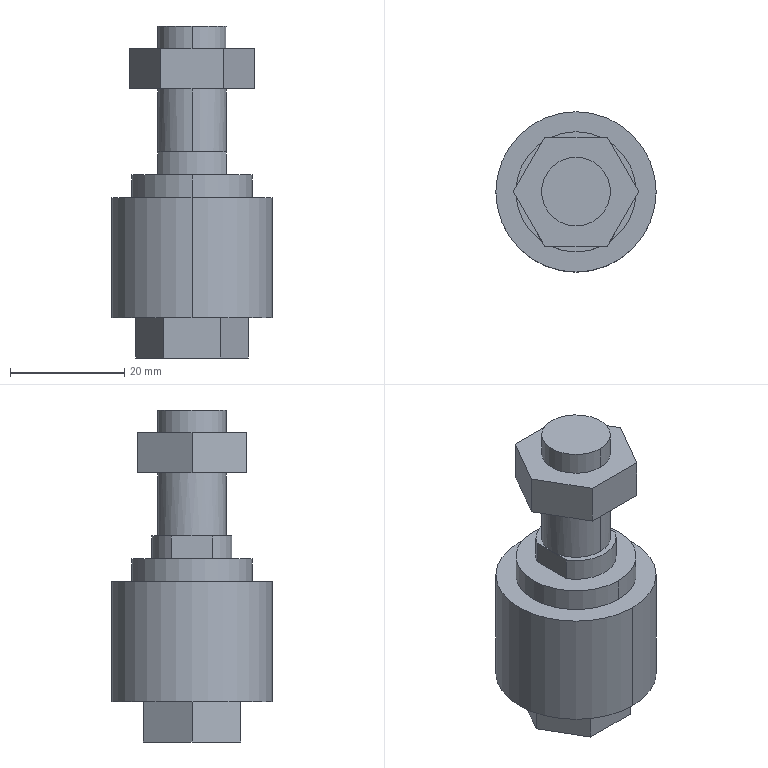Part | SolidWorks | features BaseBody 1 | 1 solid | 37 faces | box 28 x 28 x 58 mm | volume 19476 mm3 | plane 24 | cylinder 13 | commonest cylinder face diameters 12 x4 14 x3 10.8 x2 21 x2 28 x2
STEP:
#1=CARTESIAN_POINT('',(-5.4,0.,11.5));
#2=VERTEX_POINT('',#1);
#3=CARTESIAN_POINT('',(5.4,0.,11.5));
#4=VERTEX_POINT('',#3);
#5=CARTESIAN_POINT('',(0.,0.,11.5));
#6=DIRECTION('',(0.,0.,-1.));
#7=DIRECTION('',(-1.,0.,0.));
#8=AXIS2_PLACEMENT_3D('',#5,#6,#7);
#9=CIRCLE('',#8,5.4);
#10=EDGE_CURVE('',#2,#4,#9,.T.);
#11=ORIENTED_EDGE('',*,*,#10,.T.);
#12=CARTESIAN_POINT('',(0.,0.,11.5));
#13=DIRECTION('',(0.,0.,-1.));
#14=DIRECTION('',(-1.,0.,0.));
#15=AXIS2_PLACEMENT_3D('',#12,#13,#14);
#16=CIRCLE('',#15,5.4);
#17=EDGE_CURVE('',#4,#2,#16,.T.);
#18=ORIENTED_EDGE('',*,*,#17,.T.);
#19=EDGE_LOOP('',(#11,#18));
#20=FACE_OUTER_BOUND('',#19,.T.);
#21=CARTESIAN_POINT('',(0.,0.,11.5));
#22=DIRECTION('',(0.,0.,-1.));
#23=DIRECTION('',(0.,-1.,0.));
#24=AXIS2_PLACEMENT_3D('',#21,#22,#23);
#25=PLANE('',#24);
#26=ADVANCED_FACE('',(#20),#25,.T.);
#27=CARTESIAN_POINT('',(5.4,0.,0.));
#28=VERTEX_POINT('',#27);
#29=CARTESIAN_POINT('',(5.4,0.,11.5));
#30=DIRECTION('',(0.,0.,-1.));
#31=VECTOR('',#30,1000.);
#32=LINE('',#29,#31);
#33=EDGE_CURVE('',#4,#28,#32,.T.);
#34=ORIENTED_EDGE('',*,*,#33,.F.);
#35=ORIENTED_EDGE('',*,*,#10,.F.);
#36=CARTESIAN_POINT('',(-5.4,0.,0.));
#37=VERTEX_POINT('',#36);
#38=CARTESIAN_POINT('',(-5.4,0.,11.5));
#39=DIRECTION('',(0.,0.,-1.));
#40=VECTOR('',#39,1000.);
#41=LINE('',#38,#40);
#42=EDGE_CURVE('',#2,#37,#41,.T.);
#43=ORIENTED_EDGE('',*,*,#42,.T.);
#44=CARTESIAN_POINT('',(0.,0.,0.));
#45=DIRECTION('',(0.,0.,-1.));
#46=DIRECTION('',(-1.,0.,0.));
#47=AXIS2_PLACEMENT_3D('',#44,#45,#46);
#48=CIRCLE('',#47,5.4);
#49=EDGE_CURVE('',#37,#28,#48,.T.);
#50=ORIENTED_EDGE('',*,*,#49,.T.);
#51=EDGE_LOOP('',(#34,#35,#43,#50));
#52=FACE_OUTER_BOUND('',#51,.T.);
#53=CARTESIAN_POINT('',(0.,0.,11.5));
#54=DIRECTION('',(0.,0.,-1.));
#55=DIRECTION('',(-1.,0.,0.));
#56=AXIS2_PLACEMENT_3D('',#53,#54,#55);
#57=CYLINDRICAL_SURFACE('',#56,5.4);
#58=ADVANCED_FACE('',(#52),#57,.F.);
#59=CARTESIAN_POINT('',(0.,-6.,58.));
#60=VERTEX_POINT('',#59);
#61=CARTESIAN_POINT('',(0.,-6.,54.));
#62=VERTEX_POINT('',#61);
#63=CARTESIAN_POINT('',(0.,-6.,0.));
#64=DIRECTION('',(0.,0.,-1.));
#65=VECTOR('',#64,1000.);
#66=LINE('',#63,#65);
#67=EDGE_CURVE('',#60,#62,#66,.T.);
#68=ORIENTED_EDGE('',*,*,#67,.F.);
#69=CARTESIAN_POINT('',(0.,6.,58.));
#70=VERTEX_POINT('',#69);
#71=CARTESIAN_POINT('',(0.,0.,58.));
#72=DIRECTION('',(0.,0.,-1.));
#73=DIRECTION('',(0.,1.,0.));
#74=AXIS2_PLACEMENT_3D('',#71,#72,#73);
#75=CIRCLE('',#74,6.);
#76=EDGE_CURVE('',#60,#70,#75,.T.);
#77=ORIENTED_EDGE('',*,*,#76,.T.);
#78=CARTESIAN_POINT('',(0.,6.,54.));
#79=VERTEX_POINT('',#78);
#80=CARTESIAN_POINT('',(0.,6.,0.));
#81=DIRECTION('',(0.,0.,-1.));
#82=VECTOR('',#81,1000.);
#83=LINE('',#80,#82);
#84=EDGE_CURVE('',#70,#79,#83,.T.);
#85=ORIENTED_EDGE('',*,*,#84,.T.);
#86=CARTESIAN_POINT('',(0.,0.,54.));
#87=DIRECTION('',(0.,0.,-1.));
#88=DIRECTION('',(1.,0.,0.));
#89=AXIS2_PLACEMENT_3D('',#86,#87,#88);
#90=CIRCLE('',#89,6.);
#91=EDGE_CURVE('',#62,#79,#90,.T.);
#92=ORIENTED_EDGE('',*,*,#91,.F.);
#93=EDGE_LOOP('',(#68,#77,#85,#92));
#94=FACE_OUTER_BOUND('',#93,.T.);
#95=CARTESIAN_POINT('',(0.,0.,0.));
#96=DIRECTION('',(0.,0.,-1.));
#97=DIRECTION('',(0.,1.,0.));
#98=AXIS2_PLACEMENT_3D('',#95,#96,#97);
#99=CYLINDRICAL_SURFACE('',#98,6.);
#100=ADVANCED_FACE('',(#94),#99,.T.);
#101=CARTESIAN_POINT('',(0.,0.,58.));
#102=DIRECTION('',(0.,0.,-1.));
#103=DIRECTION('',(0.,1.,0.));
#104=AXIS2_PLACEMENT_3D('',#101,#102,#103);
#105=CIRCLE('',#104,6.);
#106=EDGE_CURVE('',#70,#60,#105,.T.);
#107=ORIENTED_EDGE('',*,*,#106,.F.);
#108=ORIENTED_EDGE('',*,*,#76,.F.);
#109=EDGE_LOOP('',(#107,#108));
#110=FACE_OUTER_BOUND('',#109,.T.);
#111=CARTESIAN_POINT('',(0.,6.,58.));
#112=DIRECTION('',(0.,0.,1.));
#113=DIRECTION('',(0.,-1.,0.));
#114=AXIS2_PLACEMENT_3D('',#111,#112,#113);
#115=PLANE('',#114);
#116=ADVANCED_FACE('',(#110),#115,.T.);
#117=CARTESIAN_POINT('',(0.,0.,54.));
#118=DIRECTION('',(0.,0.,-1.));
#119=DIRECTION('',(1.,0.,0.));
#120=AXIS2_PLACEMENT_3D('',#117,#118,#119);
#121=CIRCLE('',#120,6.);
#122=EDGE_CURVE('',#79,#62,#121,.T.);
#123=ORIENTED_EDGE('',*,*,#122,.T.);
#124=ORIENTED_EDGE('',*,*,#91,.T.);
#125=EDGE_LOOP('',(#123,#124));
#126=FACE_BOUND('',#125,.T.);
#127=CARTESIAN_POINT('',(-5.485,-9.5,54.));
#128=VERTEX_POINT('',#127);
#129=CARTESIAN_POINT('',(5.485,-9.5,54.));
#130=VERTEX_POINT('',#129);
#131=CARTESIAN_POINT('',(-5.485,-9.5,54.));
#132=DIRECTION('',(1.,0.,0.));
#133=VECTOR('',#132,1000.);
#134=LINE('',#131,#133);
#135=EDGE_CURVE('',#128,#130,#134,.T.);
#136=ORIENTED_EDGE('',*,*,#135,.T.);
#137=CARTESIAN_POINT('',(10.97,0.,54.));
#138=VERTEX_POINT('',#137);
#139=CARTESIAN_POINT('',(5.485,-9.5,54.));
#140=DIRECTION('',(0.5,0.866,0.));
#141=VECTOR('',#140,1000.);
#142=LINE('',#139,#141);
#143=EDGE_CURVE('',#130,#138,#142,.T.);
#144=ORIENTED_EDGE('',*,*,#143,.T.);
#145=CARTESIAN_POINT('',(5.485,9.5,54.));
#146=VERTEX_POINT('',#145);
#147=CARTESIAN_POINT('',(10.97,0.,54.));
#148=DIRECTION('',(-0.5,0.866,0.));
#149=VECTOR('',#148,1000.);
#150=LINE('',#147,#149);
#151=EDGE_CURVE('',#138,#146,#150,.T.);
#152=ORIENTED_EDGE('',*,*,#151,.T.);
#153=CARTESIAN_POINT('',(-5.485,9.5,54.));
#154=VERTEX_POINT('',#153);
#155=CARTESIAN_POINT('',(5.485,9.5,54.));
#156=DIRECTION('',(-1.,0.,0.));
#157=VECTOR('',#156,1000.);
#158=LINE('',#155,#157);
#159=EDGE_CURVE('',#146,#154,#158,.T.);
#160=ORIENTED_EDGE('',*,*,#159,.T.);
#161=CARTESIAN_POINT('',(-10.97,0.,54.));
#162=VERTEX_POINT('',#161);
#163=CARTESIAN_POINT('',(-5.485,9.5,54.));
#164=DIRECTION('',(-0.5,-0.866,0.));
#165=VECTOR('',#164,1000.);
#166=LINE('',#163,#165);
#167=EDGE_CURVE('',#154,#162,#166,.T.);
#168=ORIENTED_EDGE('',*,*,#167,.T.);
#169=CARTESIAN_POINT('',(-10.97,0.,54.));
#170=DIRECTION('',(0.5,-0.866,0.));
#171=VECTOR('',#170,1000.);
#172=LINE('',#169,#171);
#173=EDGE_CURVE('',#162,#128,#172,.T.);
#174=ORIENTED_EDGE('',*,*,#173,.T.);
#175=EDGE_LOOP('',(#136,#144,#152,#160,#168,#174));
#176=FACE_OUTER_BOUND('',#175,.T.);
#177=CARTESIAN_POINT('',(0.,0.,54.));
#178=DIRECTION('',(0.,0.,1.));
#179=DIRECTION('',(1.,0.,0.));
#180=AXIS2_PLACEMENT_3D('',#177,#178,#179);
#181=PLANE('',#180);
#182=ADVANCED_FACE('',(#126,#176),#181,.T.);
#183=CARTESIAN_POINT('',(0.,6.,47.));
#184=VERTEX_POINT('',#183);
#185=CARTESIAN_POINT('',(0.,-6.,47.));
#186=VERTEX_POINT('',#185);
#187=CARTESIAN_POINT('',(0.,0.,47.));
#188=DIRECTION('',(0.,0.,-1.));
#189=DIRECTION('',(1.,0.,0.));
#190=AXIS2_PLACEMENT_3D('',#187,#188,#189);
#191=CIRCLE('',#190,6.);
#192=EDGE_CURVE('',#184,#186,#191,.T.);
#193=ORIENTED_EDGE('',*,*,#192,.F.);
#194=CARTESIAN_POINT('',(0.,0.,47.));
#195=DIRECTION('',(0.,0.,-1.));
#196=DIRECTION('',(1.,0.,0.));
#197=AXIS2_PLACEMENT_3D('',#194,#195,#196);
#198=CIRCLE('',#197,6.);
#199=EDGE_CURVE('',#186,#184,#198,.T.);
#200=ORIENTED_EDGE('',*,*,#199,.F.);
#201=EDGE_LOOP('',(#193,#200));
#202=FACE_BOUND('',#201,.T.);
#203=CARTESIAN_POINT('',(-5.485,-9.5,47.));
#204=VERTEX_POINT('',#203);
#205=CARTESIAN_POINT('',(5.485,-9.5,47.));
#206=VERTEX_POINT('',#205);
#207=CARTESIAN_POINT('',(-5.485,-9.5,47.));
#208=DIRECTION('',(1.,0.,0.));
#209=VECTOR('',#208,1000.);
#210=LINE('',#207,#209);
#211=EDGE_CURVE('',#204,#206,#210,.T.);
#212=ORIENTED_EDGE('',*,*,#211,.F.);
#213=CARTESIAN_POINT('',(-10.97,0.,47.));
#214=VERTEX_POINT('',#213);
#215=CARTESIAN_POINT('',(-10.97,0.,47.));
#216=DIRECTION('',(0.5,-0.866,0.));
#217=VECTOR('',#216,1000.);
#218=LINE('',#215,#217);
#219=EDGE_CURVE('',#214,#204,#218,.T.);
#220=ORIENTED_EDGE('',*,*,#219,.F.);
#221=CARTESIAN_POINT('',(-5.485,9.5,47.));
#222=VERTEX_POINT('',#221);
#223=CARTESIAN_POINT('',(-5.485,9.5,47.));
#224=DIRECTION('',(-0.5,-0.866,0.));
#225=VECTOR('',#224,1000.);
#226=LINE('',#223,#225);
#227=EDGE_CURVE('',#222,#214,#226,.T.);
#228=ORIENTED_EDGE('',*,*,#227,.F.);
#229=CARTESIAN_POINT('',(5.485,9.5,47.));
#230=VERTEX_POINT('',#229);
#231=CARTESIAN_POINT('',(5.485,9.5,47.));
#232=DIRECTION('',(-1.,0.,0.));
#233=VECTOR('',#232,1000.);
#234=LINE('',#231,#233);
#235=EDGE_CURVE('',#230,#222,#234,.T.);
#236=ORIENTED_EDGE('',*,*,#235,.F.);
#237=CARTESIAN_POINT('',(10.97,0.,47.));
#238=VERTEX_POINT('',#237);
#239=CARTESIAN_POINT('',(10.97,0.,47.));
#240=DIRECTION('',(-0.5,0.866,0.));
#241=VECTOR('',#240,1000.);
#242=LINE('',#239,#241);
#243=EDGE_CURVE('',#238,#230,#242,.T.);
#244=ORIENTED_EDGE('',*,*,#243,.F.);
#245=CARTESIAN_POINT('',(5.485,-9.5,47.));
#246=DIRECTION('',(0.5,0.866,0.));
#247=VECTOR('',#246,1000.);
#248=LINE('',#245,#247);
#249=EDGE_CURVE('',#206,#238,#248,.T.);
#250=ORIENTED_EDGE('',*,*,#249,.F.);
#251=EDGE_LOOP('',(#212,#220,#228,#236,#244,#250));
#252=FACE_OUTER_BOUND('',#251,.T.);
#253=CARTESIAN_POINT('',(0.,0.,47.));
#254=DIRECTION('',(0.,0.,1.));
#255=DIRECTION('',(1.,0.,0.));
#256=AXIS2_PLACEMENT_3D('',#253,#254,#255);
#257=PLANE('',#256);
#258=ADVANCED_FACE('',(#202,#252),#257,.F.);
#259=ORIENTED_EDGE('',*,*,#143,.F.);
#260=CARTESIAN_POINT('',(5.485,-9.5,47.));
#261=DIRECTION('',(0.,0.,1.));
#262=VECTOR('',#261,1000.);
#263=LINE('',#260,#262);
#264=EDGE_CURVE('',#206,#130,#263,.T.);
#265=ORIENTED_EDGE('',*,*,#264,.F.);
#266=ORIENTED_EDGE('',*,*,#249,.T.);
#267=CARTESIAN_POINT('',(10.97,0.,47.));
#268=DIRECTION('',(0.,0.,1.));
#269=VECTOR('',#268,1000.);
#270=LINE('',#267,#269);
#271=EDGE_CURVE('',#238,#138,#270,.T.);
#272=ORIENTED_EDGE('',*,*,#271,.T.);
#273=EDGE_LOOP('',(#259,#265,#266,#272));
#274=FACE_OUTER_BOUND('',#273,.T.);
#275=CARTESIAN_POINT('',(5.485,-9.5,47.));
#276=DIRECTION('',(0.866,-0.5,0.));
#277=DIRECTION('',(0.,0.,-1.));
#278=AXIS2_PLACEMENT_3D('',#275,#276,#277);
#279=PLANE('',#278);
#280=ADVANCED_FACE('',(#274),#279,.T.);
#281=ORIENTED_EDGE('',*,*,#151,.F.);
#282=ORIENTED_EDGE('',*,*,#271,.F.);
#283=ORIENTED_EDGE('',*,*,#243,.T.);
#284=CARTESIAN_POINT('',(5.485,9.5,47.));
#285=DIRECTION('',(0.,0.,1.));
#286=VECTOR('',#285,1000.);
#287=LINE('',#284,#286);
#288=EDGE_CURVE('',#230,#146,#287,.T.);
#289=ORIENTED_EDGE('',*,*,#288,.T.);
#290=EDGE_LOOP('',(#281,#282,#283,#289));
#291=FACE_OUTER_BOUND('',#290,.T.);
#292=CARTESIAN_POINT('',(10.97,0.,47.));
#293=DIRECTION('',(0.866,0.5,0.));
#294=DIRECTION('',(0.,0.,-1.));
#295=AXIS2_PLACEMENT_3D('',#292,#293,#294);
#296=PLANE('',#295);
#297=ADVANCED_FACE('',(#291),#296,.T.);
#298=ORIENTED_EDGE('',*,*,#159,.F.);
#299=ORIENTED_EDGE('',*,*,#288,.F.);
#300=ORIENTED_EDGE('',*,*,#235,.T.);
#301=CARTESIAN_POINT('',(-5.485,9.5,47.));
#302=DIRECTION('',(0.,0.,1.));
#303=VECTOR('',#302,1000.);
#304=LINE('',#301,#303);
#305=EDGE_CURVE('',#222,#154,#304,.T.);
#306=ORIENTED_EDGE('',*,*,#305,.T.);
#307=EDGE_LOOP('',(#298,#299,#300,#306));
#308=FACE_OUTER_BOUND('',#307,.T.);
#309=CARTESIAN_POINT('',(5.485,9.5,47.));
#310=DIRECTION('',(0.,1.,0.));
#311=DIRECTION('',(1.,0.,0.));
#312=AXIS2_PLACEMENT_3D('',#309,#310,#311);
#313=PLANE('',#312);
#314=ADVANCED_FACE('',(#308),#313,.T.);
#315=ORIENTED_EDGE('',*,*,#167,.F.);
#316=ORIENTED_EDGE('',*,*,#305,.F.);
#317=ORIENTED_EDGE('',*,*,#227,.T.);
#318=CARTESIAN_POINT('',(-10.97,0.,47.));
#319=DIRECTION('',(0.,0.,1.));
#320=VECTOR('',#319,1000.);
#321=LINE('',#318,#320);
#322=EDGE_CURVE('',#214,#162,#321,.T.);
#323=ORIENTED_EDGE('',*,*,#322,.T.);
#324=EDGE_LOOP('',(#315,#316,#317,#323));
#325=FACE_OUTER_BOUND('',#324,.T.);
#326=CARTESIAN_POINT('',(-5.485,9.5,47.));
#327=DIRECTION('',(-0.866,0.5,0.));
#328=DIRECTION('',(0.,0.,1.));
#329=AXIS2_PLACEMENT_3D('',#326,#327,#328);
#330=PLANE('',#329);
#331=ADVANCED_FACE('',(#325),#330,.T.);
#332=ORIENTED_EDGE('',*,*,#173,.F.);
#333=ORIENTED_EDGE('',*,*,#322,.F.);
#334=ORIENTED_EDGE('',*,*,#219,.T.);
#335=CARTESIAN_POINT('',(-5.485,-9.5,47.));
#336=DIRECTION('',(0.,0.,1.));
#337=VECTOR('',#336,1000.);
#338=LINE('',#335,#337);
#339=EDGE_CURVE('',#204,#128,#338,.T.);
#340=ORIENTED_EDGE('',*,*,#339,.T.);
#341=EDGE_LOOP('',(#332,#333,#334,#340));
#342=FACE_OUTER_BOUND('',#341,.T.);
#343=CARTESIAN_POINT('',(-10.97,0.,47.));
#344=DIRECTION('',(-0.866,-0.5,0.));
#345=DIRECTION('',(-0.5,0.866,0.));
#346=AXIS2_PLACEMENT_3D('',#343,#344,#345);
#347=PLANE('',#346);
#348=ADVANCED_FACE('',(#342),#347,.T.);
#349=ORIENTED_EDGE('',*,*,#135,.F.);
#350=ORIENTED_EDGE('',*,*,#339,.F.);
#351=ORIENTED_EDGE('',*,*,#211,.T.);
#352=ORIENTED_EDGE('',*,*,#264,.T.);
#353=EDGE_LOOP('',(#349,#350,#351,#352));
#354=FACE_OUTER_BOUND('',#353,.T.);
#355=CARTESIAN_POINT('',(-5.485,-9.5,47.));
#356=DIRECTION('',(0.,-1.,0.));
#357=DIRECTION('',(0.,0.,-1.));
#358=AXIS2_PLACEMENT_3D('',#355,#356,#357);
#359=PLANE('',#358);
#360=ADVANCED_FACE('',(#354),#359,.T.);
#361=CARTESIAN_POINT('',(-6.,-3.606,32.));
#362=VERTEX_POINT('',#361);
#363=CARTESIAN_POINT('',(-6.,3.606,32.));
#364=VERTEX_POINT('',#363);
#365=CARTESIAN_POINT('',(-6.,-7.,32.));
#366=DIRECTION('',(0.,1.,0.));
#367=VECTOR('',#366,1000.);
#368=LINE('',#365,#367);
#369=EDGE_CURVE('',#362,#364,#368,.T.);
#370=ORIENTED_EDGE('',*,*,#369,.F.);
#371=CARTESIAN_POINT('',(-6.,-3.606,36.));
#372=VERTEX_POINT('',#371);
#373=CARTESIAN_POINT('',(-6.,-3.606,0.));
#374=DIRECTION('',(0.,0.,-1.));
#375=VECTOR('',#374,1000.);
#376=LINE('',#373,#375);
#377=EDGE_CURVE('',#372,#362,#376,.T.);
#378=ORIENTED_EDGE('',*,*,#377,.F.);
#379=CARTESIAN_POINT('',(-6.,0.,36.));
#380=VERTEX_POINT('',#379);
#381=CARTESIAN_POINT('',(-6.,-7.,36.));
#382=DIRECTION('',(0.,-1.,0.));
#383=VECTOR('',#382,1000.);
#384=LINE('',#381,#383);
#385=EDGE_CURVE('',#380,#372,#384,.T.);
#386=ORIENTED_EDGE('',*,*,#385,.F.);
#387=CARTESIAN_POINT('',(-6.,3.606,36.));
#388=VERTEX_POINT('',#387);
#389=CARTESIAN_POINT('',(-6.,-7.,36.));
#390=DIRECTION('',(0.,-1.,0.));
#391=VECTOR('',#390,1000.);
#392=LINE('',#389,#391);
#393=EDGE_CURVE('',#388,#380,#392,.T.);
#394=ORIENTED_EDGE('',*,*,#393,.F.);
#395=CARTESIAN_POINT('',(-6.,3.606,0.));
#396=DIRECTION('',(0.,0.,1.));
#397=VECTOR('',#396,1000.);
#398=LINE('',#395,#397);
#399=EDGE_CURVE('',#364,#388,#398,.T.);
#400=ORIENTED_EDGE('',*,*,#399,.F.);
#401=EDGE_LOOP('',(#370,#378,#386,#394,#400));
#402=FACE_OUTER_BOUND('',#401,.T.);
#403=CARTESIAN_POINT('',(-6.,-7.,-7.994));
#404=DIRECTION('',(-1.,0.,0.));
#405=DIRECTION('',(0.,0.,1.));
#406=AXIS2_PLACEMENT_3D('',#403,#404,#405);
#407=PLANE('',#406);
#408=ADVANCED_FACE('',(#402),#407,.T.);
#409=CARTESIAN_POINT('',(6.,3.606,32.));
#410=VERTEX_POINT('',#409);
#411=CARTESIAN_POINT('',(6.,-3.606,32.));
#412=VERTEX_POINT('',#411);
#413=CARTESIAN_POINT('',(6.,-7.,32.));
#414=DIRECTION('',(0.,-1.,0.));
#415=VECTOR('',#414,1000.);
#416=LINE('',#413,#415);
#417=EDGE_CURVE('',#410,#412,#416,.T.);
#418=ORIENTED_EDGE('',*,*,#417,.F.);
#419=CARTESIAN_POINT('',(6.,3.606,36.));
#420=VERTEX_POINT('',#419);
#421=CARTESIAN_POINT('',(6.,3.606,0.));
#422=DIRECTION('',(0.,0.,-1.));
#423=VECTOR('',#422,1000.);
#424=LINE('',#421,#423);
#425=EDGE_CURVE('',#420,#410,#424,.T.);
#426=ORIENTED_EDGE('',*,*,#425,.F.);
#427=CARTESIAN_POINT('',(6.,0.,36.));
#428=VERTEX_POINT('',#427);
#429=CARTESIAN_POINT('',(6.,-7.,36.));
#430=DIRECTION('',(0.,1.,0.));
#431=VECTOR('',#430,1000.);
#432=LINE('',#429,#431);
#433=EDGE_CURVE('',#428,#420,#432,.T.);
#434=ORIENTED_EDGE('',*,*,#433,.F.);
#435=CARTESIAN_POINT('',(6.,-3.606,36.));
#436=VERTEX_POINT('',#435);
#437=CARTESIAN_POINT('',(6.,-7.,36.));
#438=DIRECTION('',(0.,1.,0.));
#439=VECTOR('',#438,1000.);
#440=LINE('',#437,#439);
#441=EDGE_CURVE('',#436,#428,#440,.T.);
#442=ORIENTED_EDGE('',*,*,#441,.F.);
#443=CARTESIAN_POINT('',(6.,-3.606,0.));
#444=DIRECTION('',(0.,0.,1.));
#445=VECTOR('',#444,1000.);
#446=LINE('',#443,#445);
#447=EDGE_CURVE('',#412,#436,#446,.T.);
#448=ORIENTED_EDGE('',*,*,#447,.F.);
#449=EDGE_LOOP('',(#418,#426,#434,#442,#448));
#450=FACE_OUTER_BOUND('',#449,.T.);
#451=CARTESIAN_POINT('',(6.,-7.,-7.994));
#452=DIRECTION('',(1.,0.,0.));
#453=DIRECTION('',(0.,1.,0.));
#454=AXIS2_PLACEMENT_3D('',#451,#452,#453);
#455=PLANE('',#454);
#456=ADVANCED_FACE('',(#450),#455,.T.);
#457=ORIENTED_EDGE('',*,*,#369,.T.);
#458=CARTESIAN_POINT('',(0.,7.,32.));
#459=VERTEX_POINT('',#458);
#460=CARTESIAN_POINT('',(0.,0.,32.));
#461=DIRECTION('',(0.,0.,-1.));
#462=DIRECTION('',(0.,1.,0.));
#463=AXIS2_PLACEMENT_3D('',#460,#461,#462);
#464=CIRCLE('',#463,7.);
#465=EDGE_CURVE('',#364,#459,#464,.T.);
#466=ORIENTED_EDGE('',*,*,#465,.T.);
#467=CARTESIAN_POINT('',(0.,0.,32.));
#468=DIRECTION('',(0.,0.,-1.));
#469=DIRECTION('',(0.,1.,0.));
#470=AXIS2_PLACEMENT_3D('',#467,#468,#469);
#471=CIRCLE('',#470,7.);
#472=EDGE_CURVE('',#459,#410,#471,.T.);
#473=ORIENTED_EDGE('',*,*,#472,.T.);
#474=ORIENTED_EDGE('',*,*,#417,.T.);
#475=CARTESIAN_POINT('',(0.,0.,32.));
#476=DIRECTION('',(0.,0.,-1.));
#477=DIRECTION('',(0.,1.,0.));
#478=AXIS2_PLACEMENT_3D('',#475,#476,#477);
#479=CIRCLE('',#478,7.);
#480=EDGE_CURVE('',#412,#362,#479,.T.);
#481=ORIENTED_EDGE('',*,*,#480,.T.);
#482=EDGE_LOOP('',(#457,#466,#473,#474,#481));
#483=FACE_BOUND('',#482,.T.);
#484=CARTESIAN_POINT('',(0.,10.5,32.));
#485=VERTEX_POINT('',#484);
#486=CARTESIAN_POINT('',(0.,-10.5,32.));
#487=VERTEX_POINT('',#486);
#488=CARTESIAN_POINT('',(0.,0.,32.));
#489=DIRECTION('',(0.,0.,-1.));
#490=DIRECTION('',(0.,1.,0.));
#491=AXIS2_PLACEMENT_3D('',#488,#489,#490);
#492=CIRCLE('',#491,10.5);
#493=EDGE_CURVE('',#485,#487,#492,.T.);
#494=ORIENTED_EDGE('',*,*,#493,.F.);
#495=CARTESIAN_POINT('',(0.,0.,32.));
#496=DIRECTION('',(0.,0.,-1.));
#497=DIRECTION('',(0.,1.,0.));
#498=AXIS2_PLACEMENT_3D('',#495,#496,#497);
#499=CIRCLE('',#498,10.5);
#500=EDGE_CURVE('',#487,#485,#499,.T.);
#501=ORIENTED_EDGE('',*,*,#500,.F.);
#502=EDGE_LOOP('',(#494,#501));
#503=FACE_OUTER_BOUND('',#502,.T.);
#504=CARTESIAN_POINT('',(0.,10.5,32.));
#505=DIRECTION('',(0.,0.,1.));
#506=DIRECTION('',(0.,-1.,0.));
#507=AXIS2_PLACEMENT_3D('',#504,#505,#506);
#508=PLANE('',#507);
#509=ADVANCED_FACE('',(#483,#503),#508,.T.);
#510=CARTESIAN_POINT('',(0.,-10.5,28.));
#511=VERTEX_POINT('',#510);
#512=CARTESIAN_POINT('',(0.,-10.5,0.));
#513=DIRECTION('',(0.,0.,-1.));
#514=VECTOR('',#513,1000.);
#515=LINE('',#512,#514);
#516=EDGE_CURVE('',#487,#511,#515,.T.);
#517=ORIENTED_EDGE('',*,*,#516,.F.);
#518=ORIENTED_EDGE('',*,*,#500,.T.);
#519=CARTESIAN_POINT('',(0.,10.5,28.));
#520=VERTEX_POINT('',#519);
#521=CARTESIAN_POINT('',(0.,10.5,0.));
#522=DIRECTION('',(0.,0.,-1.));
#523=VECTOR('',#522,1000.);
#524=LINE('',#521,#523);
#525=EDGE_CURVE('',#485,#520,#524,.T.);
#526=ORIENTED_EDGE('',*,*,#525,.T.);
#527=CARTESIAN_POINT('',(0.,0.,28.));
#528=DIRECTION('',(0.,0.,-1.));
#529=DIRECTION('',(0.,1.,0.));
#530=AXIS2_PLACEMENT_3D('',#527,#528,#529);
#531=CIRCLE('',#530,10.5);
#532=EDGE_CURVE('',#511,#520,#531,.T.);
#533=ORIENTED_EDGE('',*,*,#532,.F.);
#534=EDGE_LOOP('',(#517,#518,#526,#533));
#535=FACE_OUTER_BOUND('',#534,.T.);
#536=CARTESIAN_POINT('',(0.,0.,0.));
#537=DIRECTION('',(0.,0.,-1.));
#538=DIRECTION('',(0.,1.,0.));
#539=AXIS2_PLACEMENT_3D('',#536,#537,#538);
#540=CYLINDRICAL_SURFACE('',#539,10.5);
#541=ADVANCED_FACE('',(#535),#540,.T.);
#542=CARTESIAN_POINT('',(0.,0.,28.));
#543=DIRECTION('',(0.,0.,-1.));
#544=DIRECTION('',(0.,1.,0.));
#545=AXIS2_PLACEMENT_3D('',#542,#543,#544);
#546=CIRCLE('',#545,10.5);
#547=EDGE_CURVE('',#520,#511,#546,.T.);
#548=ORIENTED_EDGE('',*,*,#547,.T.);
#549=ORIENTED_EDGE('',*,*,#532,.T.);
#550=EDGE_LOOP('',(#548,#549));
#551=FACE_BOUND('',#550,.T.);
#552=CARTESIAN_POINT('',(0.,14.,28.));
#553=VERTEX_POINT('',#552);
#554=CARTESIAN_POINT('',(0.,-14.,28.));
#555=VERTEX_POINT('',#554);
#556=CARTESIAN_POINT('',(0.,0.,28.));
#557=DIRECTION('',(0.,0.,-1.));
#558=DIRECTION('',(0.,1.,0.));
#559=AXIS2_PLACEMENT_3D('',#556,#557,#558);
#560=CIRCLE('',#559,14.);
#561=EDGE_CURVE('',#553,#555,#560,.T.);
#562=ORIENTED_EDGE('',*,*,#561,.F.);
#563=CARTESIAN_POINT('',(0.,0.,28.));
#564=DIRECTION('',(0.,0.,-1.));
#565=DIRECTION('',(0.,1.,0.));
#566=AXIS2_PLACEMENT_3D('',#563,#564,#565);
#567=CIRCLE('',#566,14.);
#568=EDGE_CURVE('',#555,#553,#567,.T.);
#569=ORIENTED_EDGE('',*,*,#568,.F.);
#570=EDGE_LOOP('',(#562,#569));
#571=FACE_OUTER_BOUND('',#570,.T.);
#572=CARTESIAN_POINT('',(0.,14.,28.));
#573=DIRECTION('',(0.,0.,1.));
#574=DIRECTION('',(0.,-1.,0.));
#575=AXIS2_PLACEMENT_3D('',#572,#573,#574);
#576=PLANE('',#575);
#577=ADVANCED_FACE('',(#551,#571),#576,.T.);
#578=CARTESIAN_POINT('',(0.,-14.,7.));
#579=VERTEX_POINT('',#578);
#580=CARTESIAN_POINT('',(0.,-14.,0.));
#581=DIRECTION('',(0.,0.,-1.));
#582=VECTOR('',#581,1000.);
#583=LINE('',#580,#582);
#584=EDGE_CURVE('',#555,#579,#583,.T.);
#585=ORIENTED_EDGE('',*,*,#584,.F.);
#586=ORIENTED_EDGE('',*,*,#568,.T.);
#587=CARTESIAN_POINT('',(0.,14.,7.));
#588=VERTEX_POINT('',#587);
#589=CARTESIAN_POINT('',(0.,14.,0.));
#590=DIRECTION('',(0.,0.,-1.));
#591=VECTOR('',#590,1000.);
#592=LINE('',#589,#591);
#593=EDGE_CURVE('',#553,#588,#592,.T.);
#594=ORIENTED_EDGE('',*,*,#593,.T.);
#595=CARTESIAN_POINT('',(0.,0.,7.));
#596=DIRECTION('',(0.,0.,-1.));
#597=DIRECTION('',(0.,1.,0.));
#598=AXIS2_PLACEMENT_3D('',#595,#596,#597);
#599=CIRCLE('',#598,14.);
#600=EDGE_CURVE('',#579,#588,#599,.T.);
#601=ORIENTED_EDGE('',*,*,#600,.F.);
#602=EDGE_LOOP('',(#585,#586,#594,#601));
#603=FACE_OUTER_BOUND('',#602,.T.);
#604=CARTESIAN_POINT('',(0.,0.,0.));
#605=DIRECTION('',(0.,0.,-1.));
#606=DIRECTION('',(0.,1.,0.));
#607=AXIS2_PLACEMENT_3D('',#604,#605,#606);
#608=CYLINDRICAL_SURFACE('',#607,14.);
#609=ADVANCED_FACE('',(#603),#608,.T.);
#610=CARTESIAN_POINT('',(-4.907,-8.5,7.));
#611=VERTEX_POINT('',#610);
#612=CARTESIAN_POINT('',(4.907,-8.5,7.));
#613=VERTEX_POINT('',#612);
#614=CARTESIAN_POINT('',(-4.907,-8.5,7.));
#615=DIRECTION('',(1.,0.,0.));
#616=VECTOR('',#615,1000.);
#617=LINE('',#614,#616);
#618=EDGE_CURVE('',#611,#613,#617,.T.);
#619=ORIENTED_EDGE('',*,*,#618,.T.);
#620=CARTESIAN_POINT('',(9.815,0.,7.));
#621=VERTEX_POINT('',#620);
#622=CARTESIAN_POINT('',(4.907,-8.5,7.));
#623=DIRECTION('',(0.5,0.866,0.));
#624=VECTOR('',#623,1000.);
#625=LINE('',#622,#624);
#626=EDGE_CURVE('',#613,#621,#625,.T.);
#627=ORIENTED_EDGE('',*,*,#626,.T.);
#628=CARTESIAN_POINT('',(4.907,8.5,7.));
#629=VERTEX_POINT('',#628);
#630=CARTESIAN_POINT('',(9.815,0.,7.));
#631=DIRECTION('',(-0.5,0.866,0.));
#632=VECTOR('',#631,1000.);
#633=LINE('',#630,#632);
#634=EDGE_CURVE('',#621,#629,#633,.T.);
#635=ORIENTED_EDGE('',*,*,#634,.T.);
#636=CARTESIAN_POINT('',(-4.907,8.5,7.));
#637=VERTEX_POINT('',#636);
#638=CARTESIAN_POINT('',(4.907,8.5,7.));
#639=DIRECTION('',(-1.,0.,0.));
#640=VECTOR('',#639,1000.);
#641=LINE('',#638,#640);
#642=EDGE_CURVE('',#629,#637,#641,.T.);
#643=ORIENTED_EDGE('',*,*,#642,.T.);
#644=CARTESIAN_POINT('',(-9.815,0.,7.));
#645=VERTEX_POINT('',#644);
#646=CARTESIAN_POINT('',(-4.907,8.5,7.));
#647=DIRECTION('',(-0.5,-0.866,0.));
#648=VECTOR('',#647,1000.);
#649=LINE('',#646,#648);
#650=EDGE_CURVE('',#637,#645,#649,.T.);
#651=ORIENTED_EDGE('',*,*,#650,.T.);
#652=CARTESIAN_POINT('',(-9.815,0.,7.));
#653=DIRECTION('',(0.5,-0.866,0.));
#654=VECTOR('',#653,1000.);
#655=LINE('',#652,#654);
#656=EDGE_CURVE('',#645,#611,#655,.T.);
#657=ORIENTED_EDGE('',*,*,#656,.T.);
#658=EDGE_LOOP('',(#619,#627,#635,#643,#651,#657));
#659=FACE_BOUND('',#658,.T.);
#660=CARTESIAN_POINT('',(0.,0.,7.));
#661=DIRECTION('',(0.,0.,-1.));
#662=DIRECTION('',(0.,1.,0.));
#663=AXIS2_PLACEMENT_3D('',#660,#661,#662);
#664=CIRCLE('',#663,14.);
#665=EDGE_CURVE('',#588,#579,#664,.T.);
#666=ORIENTED_EDGE('',*,*,#665,.T.);
#667=ORIENTED_EDGE('',*,*,#600,.T.);
#668=EDGE_LOOP('',(#666,#667));
#669=FACE_OUTER_BOUND('',#668,.T.);
#670=CARTESIAN_POINT('',(0.,0.,7.));
#671=DIRECTION('',(0.,0.,-1.));
#672=DIRECTION('',(-1.,0.,0.));
#673=AXIS2_PLACEMENT_3D('',#670,#671,#672);
#674=PLANE('',#673);
#675=ADVANCED_FACE('',(#659,#669),#674,.T.);
#676=ORIENTED_EDGE('',*,*,#49,.F.);
#677=CARTESIAN_POINT('',(0.,0.,0.));
#678=DIRECTION('',(0.,0.,-1.));
#679=DIRECTION('',(-1.,0.,0.));
#680=AXIS2_PLACEMENT_3D('',#677,#678,#679);
#681=CIRCLE('',#680,5.4);
#682=EDGE_CURVE('',#28,#37,#681,.T.);
#683=ORIENTED_EDGE('',*,*,#682,.F.);
#684=EDGE_LOOP('',(#676,#683));
#685=FACE_BOUND('',#684,.T.);
#686=CARTESIAN_POINT('',(-4.907,-8.5,0.));
#687=VERTEX_POINT('',#686);
#688=CARTESIAN_POINT('',(4.907,-8.5,0.));
#689=VERTEX_POINT('',#688);
#690=CARTESIAN_POINT('',(-4.907,-8.5,0.));
#691=DIRECTION('',(1.,0.,0.));
#692=VECTOR('',#691,1000.);
#693=LINE('',#690,#692);
#694=EDGE_CURVE('',#687,#689,#693,.T.);
#695=ORIENTED_EDGE('',*,*,#694,.F.);
#696=CARTESIAN_POINT('',(-9.815,0.,0.));
#697=VERTEX_POINT('',#696);
#698=CARTESIAN_POINT('',(-9.815,0.,0.));
#699=DIRECTION('',(0.5,-0.866,0.));
#700=VECTOR('',#699,1000.);
#701=LINE('',#698,#700);
#702=EDGE_CURVE('',#697,#687,#701,.T.);
#703=ORIENTED_EDGE('',*,*,#702,.F.);
#704=CARTESIAN_POINT('',(-4.907,8.5,0.));
#705=VERTEX_POINT('',#704);
#706=CARTESIAN_POINT('',(-4.907,8.5,0.));
#707=DIRECTION('',(-0.5,-0.866,0.));
#708=VECTOR('',#707,1000.);
#709=LINE('',#706,#708);
#710=EDGE_CURVE('',#705,#697,#709,.T.);
#711=ORIENTED_EDGE('',*,*,#710,.F.);
#712=CARTESIAN_POINT('',(4.907,8.5,0.));
#713=VERTEX_POINT('',#712);
#714=CARTESIAN_POINT('',(4.907,8.5,0.));
#715=DIRECTION('',(-1.,0.,0.));
#716=VECTOR('',#715,1000.);
#717=LINE('',#714,#716);
#718=EDGE_CURVE('',#713,#705,#717,.T.);
#719=ORIENTED_EDGE('',*,*,#718,.F.);
#720=CARTESIAN_POINT('',(9.815,0.,0.));
#721=VERTEX_POINT('',#720);
#722=CARTESIAN_POINT('',(9.815,0.,0.));
#723=DIRECTION('',(-0.5,0.866,0.));
#724=VECTOR('',#723,1000.);
#725=LINE('',#722,#724);
#726=EDGE_CURVE('',#721,#713,#725,.T.);
#727=ORIENTED_EDGE('',*,*,#726,.F.);
#728=CARTESIAN_POINT('',(4.907,-8.5,0.));
#729=DIRECTION('',(0.5,0.866,0.));
#730=VECTOR('',#729,1000.);
#731=LINE('',#728,#730);
#732=EDGE_CURVE('',#689,#721,#731,.T.);
#733=ORIENTED_EDGE('',*,*,#732,.F.);
#734=EDGE_LOOP('',(#695,#703,#711,#719,#727,#733));
#735=FACE_OUTER_BOUND('',#734,.T.);
#736=CARTESIAN_POINT('',(0.,0.,0.));
#737=DIRECTION('',(0.,0.,1.));
#738=DIRECTION('',(1.,0.,0.));
#739=AXIS2_PLACEMENT_3D('',#736,#737,#738);
#740=PLANE('',#739);
#741=ADVANCED_FACE('',(#685,#735),#740,.F.);
#742=ORIENTED_EDGE('',*,*,#702,.T.);
#743=CARTESIAN_POINT('',(-4.907,-8.5,7.));
#744=DIRECTION('',(0.,0.,-1.));
#745=VECTOR('',#744,1000.);
#746=LINE('',#743,#745);
#747=EDGE_CURVE('',#611,#687,#746,.T.);
#748=ORIENTED_EDGE('',*,*,#747,.F.);
#749=ORIENTED_EDGE('',*,*,#656,.F.);
#750=CARTESIAN_POINT('',(-9.815,0.,7.));
#751=DIRECTION('',(0.,0.,-1.));
#752=VECTOR('',#751,1000.);
#753=LINE('',#750,#752);
#754=EDGE_CURVE('',#645,#697,#753,.T.);
#755=ORIENTED_EDGE('',*,*,#754,.T.);
#756=EDGE_LOOP('',(#742,#748,#749,#755));
#757=FACE_OUTER_BOUND('',#756,.T.);
#758=CARTESIAN_POINT('',(-9.815,0.,7.));
#759=DIRECTION('',(0.866,0.5,0.));
#760=DIRECTION('',(0.,0.,-1.));
#761=AXIS2_PLACEMENT_3D('',#758,#759,#760);
#762=PLANE('',#761);
#763=ADVANCED_FACE('',(#757),#762,.F.);
#764=ORIENTED_EDGE('',*,*,#710,.T.);
#765=ORIENTED_EDGE('',*,*,#754,.F.);
#766=ORIENTED_EDGE('',*,*,#650,.F.);
#767=CARTESIAN_POINT('',(-4.907,8.5,7.));
#768=DIRECTION('',(0.,0.,-1.));
#769=VECTOR('',#768,1000.);
#770=LINE('',#767,#769);
#771=EDGE_CURVE('',#637,#705,#770,.T.);
#772=ORIENTED_EDGE('',*,*,#771,.T.);
#773=EDGE_LOOP('',(#764,#765,#766,#772));
#774=FACE_OUTER_BOUND('',#773,.T.);
#775=CARTESIAN_POINT('',(-4.907,8.5,7.));
#776=DIRECTION('',(0.866,-0.5,0.));
#777=DIRECTION('',(0.,0.,-1.));
#778=AXIS2_PLACEMENT_3D('',#775,#776,#777);
#779=PLANE('',#778);
#780=ADVANCED_FACE('',(#774),#779,.F.);
#781=ORIENTED_EDGE('',*,*,#718,.T.);
#782=ORIENTED_EDGE('',*,*,#771,.F.);
#783=ORIENTED_EDGE('',*,*,#642,.F.);
#784=CARTESIAN_POINT('',(4.907,8.5,7.));
#785=DIRECTION('',(0.,0.,-1.));
#786=VECTOR('',#785,1000.);
#787=LINE('',#784,#786);
#788=EDGE_CURVE('',#629,#713,#787,.T.);
#789=ORIENTED_EDGE('',*,*,#788,.T.);
#790=EDGE_LOOP('',(#781,#782,#783,#789));
#791=FACE_OUTER_BOUND('',#790,.T.);
#792=CARTESIAN_POINT('',(4.907,8.5,7.));
#793=DIRECTION('',(0.,-1.,0.));
#794=DIRECTION('',(0.,0.,-1.));
#795=AXIS2_PLACEMENT_3D('',#792,#793,#794);
#796=PLANE('',#795);
#797=ADVANCED_FACE('',(#791),#796,.F.);
#798=ORIENTED_EDGE('',*,*,#726,.T.);
#799=ORIENTED_EDGE('',*,*,#788,.F.);
#800=ORIENTED_EDGE('',*,*,#634,.F.);
#801=CARTESIAN_POINT('',(9.815,0.,7.));
#802=DIRECTION('',(0.,0.,-1.));
#803=VECTOR('',#802,1000.);
#804=LINE('',#801,#803);
#805=EDGE_CURVE('',#621,#721,#804,.T.);
#806=ORIENTED_EDGE('',*,*,#805,.T.);
#807=EDGE_LOOP('',(#798,#799,#800,#806));
#808=FACE_OUTER_BOUND('',#807,.T.);
#809=CARTESIAN_POINT('',(9.815,0.,7.));
#810=DIRECTION('',(-0.866,-0.5,0.));
#811=DIRECTION('',(-0.5,0.866,0.));
#812=AXIS2_PLACEMENT_3D('',#809,#810,#811);
#813=PLANE('',#812);
#814=ADVANCED_FACE('',(#808),#813,.F.);
#815=ORIENTED_EDGE('',*,*,#732,.T.);
#816=ORIENTED_EDGE('',*,*,#805,.F.);
#817=ORIENTED_EDGE('',*,*,#626,.F.);
#818=CARTESIAN_POINT('',(4.907,-8.5,7.));
#819=DIRECTION('',(0.,0.,-1.));
#820=VECTOR('',#819,1000.);
#821=LINE('',#818,#820);
#822=EDGE_CURVE('',#613,#689,#821,.T.);
#823=ORIENTED_EDGE('',*,*,#822,.T.);
#824=EDGE_LOOP('',(#815,#816,#817,#823));
#825=FACE_OUTER_BOUND('',#824,.T.);
#826=CARTESIAN_POINT('',(4.907,-8.5,7.));
#827=DIRECTION('',(-0.866,0.5,0.));
#828=DIRECTION('',(0.,0.,1.));
#829=AXIS2_PLACEMENT_3D('',#826,#827,#828);
#830=PLANE('',#829);
#831=ADVANCED_FACE('',(#825),#830,.F.);
#832=ORIENTED_EDGE('',*,*,#694,.T.);
#833=ORIENTED_EDGE('',*,*,#822,.F.);
#834=ORIENTED_EDGE('',*,*,#618,.F.);
#835=ORIENTED_EDGE('',*,*,#747,.T.);
#836=EDGE_LOOP('',(#832,#833,#834,#835));
#837=FACE_OUTER_BOUND('',#836,.T.);
#838=CARTESIAN_POINT('',(-4.907,-8.5,7.));
#839=DIRECTION('',(0.,1.,0.));
#840=DIRECTION('',(1.,0.,0.));
#841=AXIS2_PLACEMENT_3D('',#838,#839,#840);
#842=PLANE('',#841);
#843=ADVANCED_FACE('',(#837),#842,.F.);
#844=CARTESIAN_POINT('',(0.,-6.,36.));
#845=VERTEX_POINT('',#844);
#846=CARTESIAN_POINT('',(0.,0.,36.));
#847=DIRECTION('',(0.,0.,-1.));
#848=DIRECTION('',(0.,1.,0.));
#849=AXIS2_PLACEMENT_3D('',#846,#847,#848);
#850=CIRCLE('',#849,6.);
#851=EDGE_CURVE('',#428,#845,#850,.T.);
#852=ORIENTED_EDGE('',*,*,#851,.T.);
#853=CARTESIAN_POINT('',(0.,0.,36.));
#854=DIRECTION('',(0.,0.,-1.));
#855=DIRECTION('',(0.,1.,0.));
#856=AXIS2_PLACEMENT_3D('',#853,#854,#855);
#857=CIRCLE('',#856,6.);
#858=EDGE_CURVE('',#845,#380,#857,.T.);
#859=ORIENTED_EDGE('',*,*,#858,.T.);
#860=ORIENTED_EDGE('',*,*,#385,.T.);
#861=CARTESIAN_POINT('',(0.,0.,36.));
#862=DIRECTION('',(0.,0.,-1.));
#863=DIRECTION('',(0.,1.,0.));
#864=AXIS2_PLACEMENT_3D('',#861,#862,#863);
#865=CIRCLE('',#864,7.);
#866=EDGE_CURVE('',#436,#372,#865,.T.);
#867=ORIENTED_EDGE('',*,*,#866,.F.);
#868=ORIENTED_EDGE('',*,*,#441,.T.);
#869=EDGE_LOOP('',(#852,#859,#860,#867,#868));
#870=FACE_OUTER_BOUND('',#869,.T.);
#871=CARTESIAN_POINT('',(0.,7.,36.));
#872=DIRECTION('',(0.,0.,1.));
#873=DIRECTION('',(0.,-1.,0.));
#874=AXIS2_PLACEMENT_3D('',#871,#872,#873);
#875=PLANE('',#874);
#876=ADVANCED_FACE('',(#870),#875,.T.);
#877=CARTESIAN_POINT('',(0.,7.,36.));
#878=VERTEX_POINT('',#877);
#879=CARTESIAN_POINT('',(0.,0.,36.));
#880=DIRECTION('',(0.,0.,-1.));
#881=DIRECTION('',(0.,1.,0.));
#882=AXIS2_PLACEMENT_3D('',#879,#880,#881);
#883=CIRCLE('',#882,7.);
#884=EDGE_CURVE('',#388,#878,#883,.T.);
#885=ORIENTED_EDGE('',*,*,#884,.F.);
#886=ORIENTED_EDGE('',*,*,#393,.T.);
#887=CARTESIAN_POINT('',(0.,6.,36.));
#888=VERTEX_POINT('',#887);
#889=CARTESIAN_POINT('',(0.,0.,36.));
#890=DIRECTION('',(0.,0.,-1.));
#891=DIRECTION('',(0.,1.,0.));
#892=AXIS2_PLACEMENT_3D('',#889,#890,#891);
#893=CIRCLE('',#892,6.);
#894=EDGE_CURVE('',#380,#888,#893,.T.);
#895=ORIENTED_EDGE('',*,*,#894,.T.);
#896=CARTESIAN_POINT('',(0.,0.,36.));
#897=DIRECTION('',(0.,0.,-1.));
#898=DIRECTION('',(0.,1.,0.));
#899=AXIS2_PLACEMENT_3D('',#896,#897,#898);
#900=CIRCLE('',#899,6.);
#901=EDGE_CURVE('',#888,#428,#900,.T.);
#902=ORIENTED_EDGE('',*,*,#901,.T.);
#903=ORIENTED_EDGE('',*,*,#433,.T.);
#904=CARTESIAN_POINT('',(0.,0.,36.));
#905=DIRECTION('',(0.,0.,-1.));
#906=DIRECTION('',(0.,1.,0.));
#907=AXIS2_PLACEMENT_3D('',#904,#905,#906);
#908=CIRCLE('',#907,7.);
#909=EDGE_CURVE('',#878,#420,#908,.T.);
#910=ORIENTED_EDGE('',*,*,#909,.F.);
#911=EDGE_LOOP('',(#885,#886,#895,#902,#903,#910));
#912=FACE_OUTER_BOUND('',#911,.T.);
#913=CARTESIAN_POINT('',(0.,7.,36.));
#914=DIRECTION('',(0.,0.,1.));
#915=DIRECTION('',(0.,-1.,0.));
#916=AXIS2_PLACEMENT_3D('',#913,#914,#915);
#917=PLANE('',#916);
#918=ADVANCED_FACE('',(#912),#917,.T.);
#919=ORIENTED_EDGE('',*,*,#866,.T.);
#920=ORIENTED_EDGE('',*,*,#377,.T.);
#921=ORIENTED_EDGE('',*,*,#480,.F.);
#922=ORIENTED_EDGE('',*,*,#447,.T.);
#923=EDGE_LOOP('',(#919,#920,#921,#922));
#924=FACE_OUTER_BOUND('',#923,.T.);
#925=CARTESIAN_POINT('',(0.,0.,0.));
#926=DIRECTION('',(0.,0.,-1.));
#927=DIRECTION('',(0.,1.,0.));
#928=AXIS2_PLACEMENT_3D('',#925,#926,#927);
#929=CYLINDRICAL_SURFACE('',#928,7.);
#930=ADVANCED_FACE('',(#924),#929,.T.);
#931=CARTESIAN_POINT('',(0.,7.,0.));
#932=DIRECTION('',(0.,0.,-1.));
#933=VECTOR('',#932,1000.);
#934=LINE('',#931,#933);
#935=EDGE_CURVE('',#878,#459,#934,.T.);
#936=ORIENTED_EDGE('',*,*,#935,.F.);
#937=ORIENTED_EDGE('',*,*,#909,.T.);
#938=ORIENTED_EDGE('',*,*,#425,.T.);
#939=ORIENTED_EDGE('',*,*,#472,.F.);
#940=EDGE_LOOP('',(#936,#937,#938,#939));
#941=FACE_OUTER_BOUND('',#940,.T.);
#942=CARTESIAN_POINT('',(0.,0.,0.));
#943=DIRECTION('',(0.,0.,-1.));
#944=DIRECTION('',(0.,1.,0.));
#945=AXIS2_PLACEMENT_3D('',#942,#943,#944);
#946=CYLINDRICAL_SURFACE('',#945,7.);
#947=ADVANCED_FACE('',(#941),#946,.T.);
#948=CARTESIAN_POINT('',(0.,-6.,0.));
#949=DIRECTION('',(0.,0.,-1.));
#950=VECTOR('',#949,1000.);
#951=LINE('',#948,#950);
#952=EDGE_CURVE('',#186,#845,#951,.T.);
#953=ORIENTED_EDGE('',*,*,#952,.F.);
#954=ORIENTED_EDGE('',*,*,#199,.T.);
#955=CARTESIAN_POINT('',(0.,6.,0.));
#956=DIRECTION('',(0.,0.,-1.));
#957=VECTOR('',#956,1000.);
#958=LINE('',#955,#957);
#959=EDGE_CURVE('',#184,#888,#958,.T.);
#960=ORIENTED_EDGE('',*,*,#959,.T.);
#961=ORIENTED_EDGE('',*,*,#894,.F.);
#962=ORIENTED_EDGE('',*,*,#858,.F.);
#963=EDGE_LOOP('',(#953,#954,#960,#961,#962));
#964=FACE_OUTER_BOUND('',#963,.T.);
#965=CARTESIAN_POINT('',(0.,0.,0.));
#966=DIRECTION('',(0.,0.,-1.));
#967=DIRECTION('',(0.,1.,0.));
#968=AXIS2_PLACEMENT_3D('',#965,#966,#967);
#969=CYLINDRICAL_SURFACE('',#968,6.);
#970=ADVANCED_FACE('',(#964),#969,.T.);
#971=ORIENTED_EDGE('',*,*,#192,.T.);
#972=ORIENTED_EDGE('',*,*,#952,.T.);
#973=ORIENTED_EDGE('',*,*,#851,.F.);
#974=ORIENTED_EDGE('',*,*,#901,.F.);
#975=ORIENTED_EDGE('',*,*,#959,.F.);
#976=EDGE_LOOP('',(#971,#972,#973,#974,#975));
#977=FACE_OUTER_BOUND('',#976,.T.);
#978=CARTESIAN_POINT('',(0.,0.,0.));
#979=DIRECTION('',(0.,0.,-1.));
#980=DIRECTION('',(0.,1.,0.));
#981=AXIS2_PLACEMENT_3D('',#978,#979,#980);
#982=CYLINDRICAL_SURFACE('',#981,6.);
#983=ADVANCED_FACE('',(#977),#982,.T.);
#984=ORIENTED_EDGE('',*,*,#884,.T.);
#985=ORIENTED_EDGE('',*,*,#935,.T.);
#986=ORIENTED_EDGE('',*,*,#465,.F.);
#987=ORIENTED_EDGE('',*,*,#399,.T.);
#988=EDGE_LOOP('',(#984,#985,#986,#987));
#989=FACE_OUTER_BOUND('',#988,.T.);
#990=CARTESIAN_POINT('',(0.,0.,0.));
#991=DIRECTION('',(0.,0.,-1.));
#992=DIRECTION('',(0.,1.,0.));
#993=AXIS2_PLACEMENT_3D('',#990,#991,#992);
#994=CYLINDRICAL_SURFACE('',#993,7.);
#995=ADVANCED_FACE('',(#989),#994,.T.);
#996=ORIENTED_EDGE('',*,*,#561,.T.);
#997=ORIENTED_EDGE('',*,*,#584,.T.);
#998=ORIENTED_EDGE('',*,*,#665,.F.);
#999=ORIENTED_EDGE('',*,*,#593,.F.);
#1000=EDGE_LOOP('',(#996,#997,#998,#999));
#1001=FACE_OUTER_BOUND('',#1000,.T.);
#1002=CARTESIAN_POINT('',(0.,0.,0.));
#1003=DIRECTION('',(0.,0.,-1.));
#1004=DIRECTION('',(0.,1.,0.));
#1005=AXIS2_PLACEMENT_3D('',#1002,#1003,#1004);
#1006=CYLINDRICAL_SURFACE('',#1005,14.);
#1007=ADVANCED_FACE('',(#1001),#1006,.T.);
#1008=ORIENTED_EDGE('',*,*,#493,.T.);
#1009=ORIENTED_EDGE('',*,*,#516,.T.);
#1010=ORIENTED_EDGE('',*,*,#547,.F.);
#1011=ORIENTED_EDGE('',*,*,#525,.F.);
#1012=EDGE_LOOP('',(#1008,#1009,#1010,#1011));
#1013=FACE_OUTER_BOUND('',#1012,.T.);
#1014=CARTESIAN_POINT('',(0.,0.,0.));
#1015=DIRECTION('',(0.,0.,-1.));
#1016=DIRECTION('',(0.,1.,0.));
#1017=AXIS2_PLACEMENT_3D('',#1014,#1015,#1016);
#1018=CYLINDRICAL_SURFACE('',#1017,10.5);
#1019=ADVANCED_FACE('',(#1013),#1018,.T.);
#1020=ORIENTED_EDGE('',*,*,#106,.T.);
#1021=ORIENTED_EDGE('',*,*,#67,.T.);
#1022=ORIENTED_EDGE('',*,*,#122,.F.);
#1023=ORIENTED_EDGE('',*,*,#84,.F.);
#1024=EDGE_LOOP('',(#1020,#1021,#1022,#1023));
#1025=FACE_OUTER_BOUND('',#1024,.T.);
#1026=CARTESIAN_POINT('',(0.,0.,0.));
#1027=DIRECTION('',(0.,0.,-1.));
#1028=DIRECTION('',(0.,1.,0.));
#1029=AXIS2_PLACEMENT_3D('',#1026,#1027,#1028);
#1030=CYLINDRICAL_SURFACE('',#1029,6.);
#1031=ADVANCED_FACE('',(#1025),#1030,.T.);
#1032=ORIENTED_EDGE('',*,*,#17,.F.);
#1033=ORIENTED_EDGE('',*,*,#33,.T.);
#1034=ORIENTED_EDGE('',*,*,#682,.T.);
#1035=ORIENTED_EDGE('',*,*,#42,.F.);
#1036=EDGE_LOOP('',(#1032,#1033,#1034,#1035));
#1037=FACE_OUTER_BOUND('',#1036,.T.);
#1038=CARTESIAN_POINT('',(0.,0.,11.5));
#1039=DIRECTION('',(0.,0.,-1.));
#1040=DIRECTION('',(-1.,0.,0.));
#1041=AXIS2_PLACEMENT_3D('',#1038,#1039,#1040);
#1042=CYLINDRICAL_SURFACE('',#1041,5.4);
#1043=ADVANCED_FACE('',(#1037),#1042,.F.);
#1044=CLOSED_SHELL('',(#26,#58,#100,#116,#182,#258,#280,#297,#314,#331,#348,#360,#408,#456,#509,#541,#577,#609,#675,#741,#763,#780,#797,#814,#831,#843,#876,#918,#930,#947,#970,#983,#995,#1007,#1019,#1031,#1043));
#1045=MANIFOLD_SOLID_BREP('',#1044);
#1046=CARTESIAN_POINT('',(0.,0.,0.));
#1047=DIRECTION('',(0.,0.,1.));
#1048=DIRECTION('',(1.,0.,0.));
#1049=AXIS2_PLACEMENT_3D('',#1046,#1047,#1048);
#1050=(LENGTH_UNIT()NAMED_UNIT(*)SI_UNIT(.MILLI.,.METRE.));
#1051=UNCERTAINTY_MEASURE_WITH_UNIT(LENGTH_MEASURE(0.00001),#1050,'','');
#1052=(NAMED_UNIT(*)PLANE_ANGLE_UNIT()SI_UNIT($,.RADIAN.));
#1053=(NAMED_UNIT(*)SI_UNIT($,.STERADIAN.)SOLID_ANGLE_UNIT());
#1054=(GEOMETRIC_REPRESENTATION_CONTEXT(3)GLOBAL_UNCERTAINTY_ASSIGNED_CONTEXT((#1051))GLOBAL_UNIT_ASSIGNED_CONTEXT((#1050,#1052,#1053))REPRESENTATION_CONTEXT('',''));
#1055=ADVANCED_BREP_SHAPE_REPRESENTATION('',(#1045,#1049),#1054);